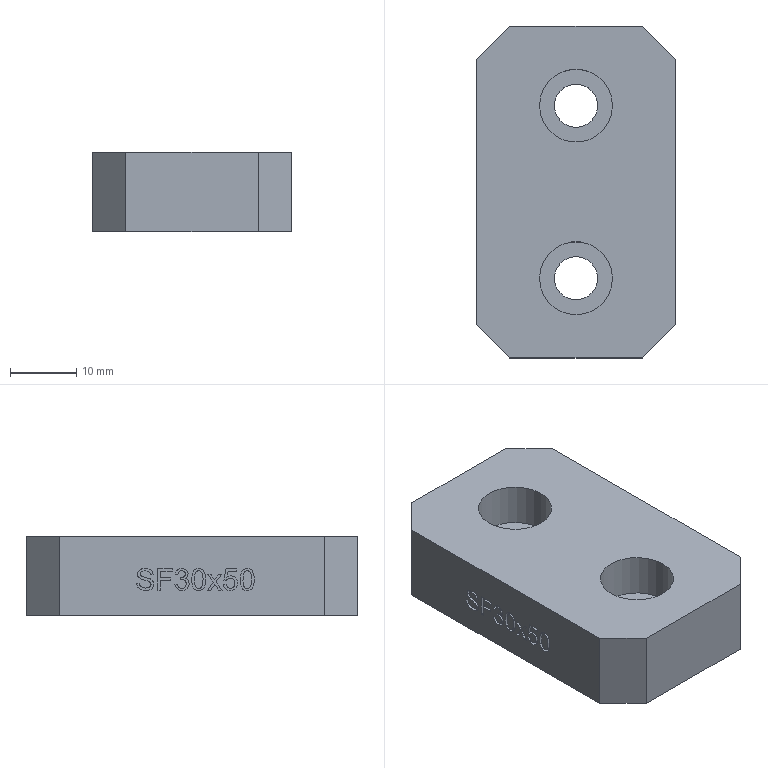Part | STEP file | lll_id366_x_t | 1 solid | 119 faces | box 30 x 50 x 12 mm | volume 15790 mm3 | other 59 | plane 56 | cylinder 4 | commonest cylinder face diameters 6.5 x2 11 x2